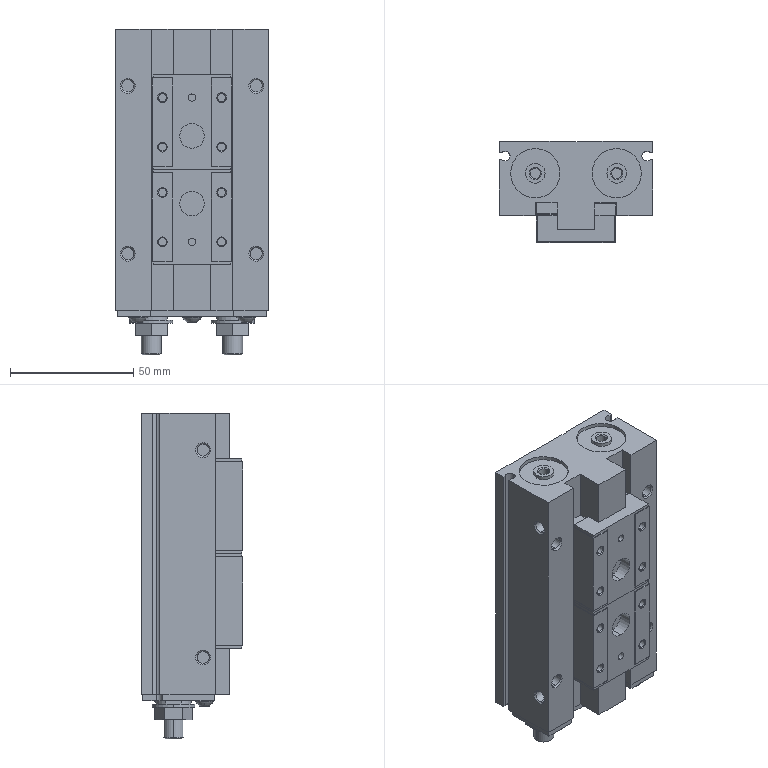Part | SolidWorks | features BaseBody 5, MoveFace 2 | 5 solids | 330 faces | box 62 x 41 x 132 mm | volume 234825 mm3 | plane 180 | cylinder 96 | cone 48 | torus 6 | commonest cylinder face diameters 4.917 x20 3.242 x16 8 x8 10 x8 5 x7 7.6 x6